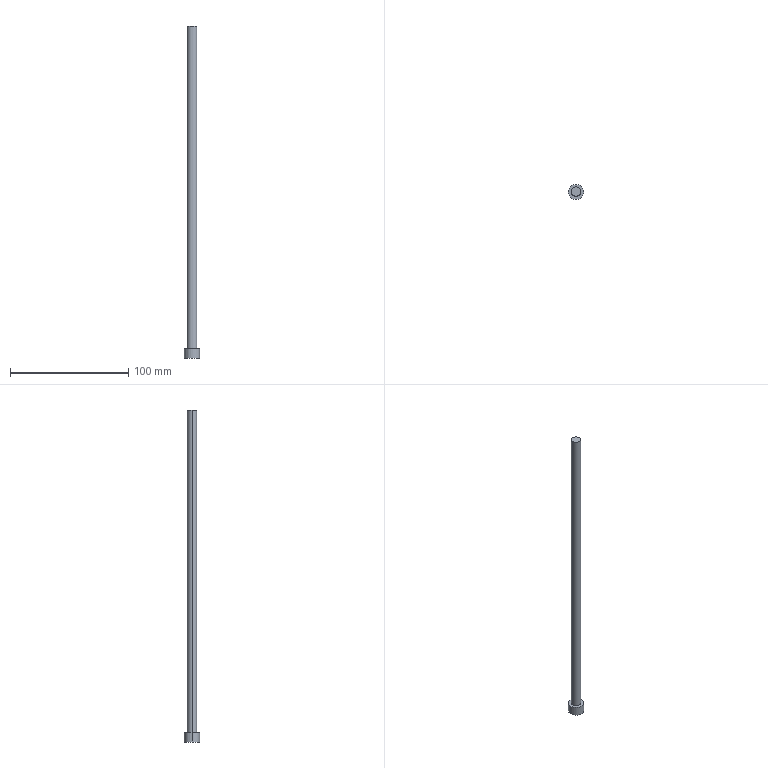Part | Creo | 1 solid | 7 faces | box 13 x 13 x 280.905 mm | volume 14780 mm3 | cylinder 4 | plane 3 | commonest cylinder face diameters 8 x2 13 x2
STEP:
#1=CARTESIAN_POINT('',(85.,64.,20.405));
#2=VERTEX_POINT('',#1);
#3=CARTESIAN_POINT('',(77.,64.,20.405));
#4=VERTEX_POINT('',#3);
#5=CARTESIAN_POINT('',(81.,64.,20.405));
#6=DIRECTION('',(0.,0.,1.));
#7=DIRECTION('',(1.,0.,0.));
#8=AXIS2_PLACEMENT_3D('',#5,#6,#7);
#9=CIRCLE('',#8,4.);
#10=EDGE_CURVE('',#2,#4,#9,.T.);
#11=ORIENTED_EDGE('',*,*,#10,.F.);
#12=CARTESIAN_POINT('',(81.,64.,20.405));
#13=DIRECTION('',(0.,0.,1.));
#14=DIRECTION('',(-1.,0.,0.));
#15=AXIS2_PLACEMENT_3D('',#12,#13,#14);
#16=CIRCLE('',#15,4.);
#17=EDGE_CURVE('',#4,#2,#16,.T.);
#18=ORIENTED_EDGE('',*,*,#17,.F.);
#19=EDGE_LOOP('',(#11,#18));
#20=FACE_OUTER_BOUND('',#19,.F.);
#21=CARTESIAN_POINT('',(81.,64.,20.405));
#22=DIRECTION('',(0.,0.,1.));
#23=DIRECTION('',(1.,0.,0.));
#24=AXIS2_PLACEMENT_3D('',#21,#22,#23);
#25=PLANE('',#24);
#26=ADVANCED_FACE('',(#20),#25,.T.);
#27=CARTESIAN_POINT('',(77.,64.,-252.5));
#28=VERTEX_POINT('',#27);
#29=CARTESIAN_POINT('',(85.,64.,-252.5));
#30=VERTEX_POINT('',#29);
#31=CARTESIAN_POINT('',(81.,64.,-252.5));
#32=DIRECTION('',(0.,0.,-1.));
#33=DIRECTION('',(-1.,0.,0.));
#34=AXIS2_PLACEMENT_3D('',#31,#32,#33);
#35=CIRCLE('',#34,4.);
#36=EDGE_CURVE('',#28,#30,#35,.T.);
#37=ORIENTED_EDGE('',*,*,#36,.T.);
#38=CARTESIAN_POINT('',(85.,64.,-252.5));
#39=DIRECTION('',(0.,0.,1.));
#40=VECTOR('',#39,272.905);
#41=LINE('',#38,#40);
#42=EDGE_CURVE('',#30,#2,#41,.T.);
#43=ORIENTED_EDGE('',*,*,#42,.T.);
#44=ORIENTED_EDGE('',*,*,#10,.T.);
#45=CARTESIAN_POINT('',(77.,64.,-252.5));
#46=DIRECTION('',(0.,0.,1.));
#47=VECTOR('',#46,272.905);
#48=LINE('',#45,#47);
#49=EDGE_CURVE('',#28,#4,#48,.T.);
#50=ORIENTED_EDGE('',*,*,#49,.F.);
#51=EDGE_LOOP('',(#37,#43,#44,#50));
#52=FACE_OUTER_BOUND('',#51,.F.);
#53=CARTESIAN_POINT('',(81.,64.,-255.5));
#54=DIRECTION('',(0.,0.,1.));
#55=DIRECTION('',(1.,0.,0.));
#56=AXIS2_PLACEMENT_3D('',#53,#54,#55);
#57=CYLINDRICAL_SURFACE('',#56,4.);
#58=ADVANCED_FACE('',(#52),#57,.T.);
#59=CARTESIAN_POINT('',(74.5,64.,-252.5));
#60=VERTEX_POINT('',#59);
#61=CARTESIAN_POINT('',(87.5,64.,-252.5));
#62=VERTEX_POINT('',#61);
#63=CARTESIAN_POINT('',(81.,64.,-252.5));
#64=DIRECTION('',(0.,0.,1.));
#65=DIRECTION('',(-1.,0.,0.));
#66=AXIS2_PLACEMENT_3D('',#63,#64,#65);
#67=CIRCLE('',#66,6.5);
#68=EDGE_CURVE('',#60,#62,#67,.T.);
#69=ORIENTED_EDGE('',*,*,#68,.F.);
#70=CARTESIAN_POINT('',(81.,64.,-252.5));
#71=DIRECTION('',(0.,0.,1.));
#72=DIRECTION('',(1.,0.,0.));
#73=AXIS2_PLACEMENT_3D('',#70,#71,#72);
#74=CIRCLE('',#73,6.5);
#75=EDGE_CURVE('',#62,#60,#74,.T.);
#76=ORIENTED_EDGE('',*,*,#75,.F.);
#77=EDGE_LOOP('',(#69,#76));
#78=FACE_OUTER_BOUND('',#77,.F.);
#79=CARTESIAN_POINT('',(81.,64.,-252.5));
#80=DIRECTION('',(0.,0.,-1.));
#81=DIRECTION('',(1.,0.,0.));
#82=AXIS2_PLACEMENT_3D('',#79,#80,#81);
#83=CIRCLE('',#82,4.);
#84=EDGE_CURVE('',#30,#28,#83,.T.);
#85=ORIENTED_EDGE('',*,*,#84,.F.);
#86=ORIENTED_EDGE('',*,*,#36,.F.);
#87=EDGE_LOOP('',(#85,#86));
#88=FACE_BOUND('',#87,.F.);
#89=CARTESIAN_POINT('',(81.,64.,-252.5));
#90=DIRECTION('',(0.,0.,1.));
#91=DIRECTION('',(1.,0.,0.));
#92=AXIS2_PLACEMENT_3D('',#89,#90,#91);
#93=PLANE('',#92);
#94=ADVANCED_FACE('',(#78,#88),#93,.T.);
#95=ORIENTED_EDGE('',*,*,#84,.T.);
#96=ORIENTED_EDGE('',*,*,#49,.T.);
#97=ORIENTED_EDGE('',*,*,#17,.T.);
#98=ORIENTED_EDGE('',*,*,#42,.F.);
#99=EDGE_LOOP('',(#95,#96,#97,#98));
#100=FACE_OUTER_BOUND('',#99,.F.);
#101=CARTESIAN_POINT('',(81.,64.,-255.5));
#102=DIRECTION('',(0.,0.,1.));
#103=DIRECTION('',(1.,0.,0.));
#104=AXIS2_PLACEMENT_3D('',#101,#102,#103);
#105=CYLINDRICAL_SURFACE('',#104,4.);
#106=ADVANCED_FACE('',(#100),#105,.T.);
#107=ORIENTED_EDGE('',*,*,#68,.T.);
#108=CARTESIAN_POINT('',(87.5,64.,-260.5));
#109=VERTEX_POINT('',#108);
#110=CARTESIAN_POINT('',(87.5,64.,-260.5));
#111=DIRECTION('',(0.,0.,1.));
#112=VECTOR('',#111,8.);
#113=LINE('',#110,#112);
#114=EDGE_CURVE('',#109,#62,#113,.T.);
#115=ORIENTED_EDGE('',*,*,#114,.F.);
#116=CARTESIAN_POINT('',(74.5,64.,-260.5));
#117=VERTEX_POINT('',#116);
#118=CARTESIAN_POINT('',(81.,64.,-260.5));
#119=DIRECTION('',(0.,0.,-1.));
#120=DIRECTION('',(1.,0.,0.));
#121=AXIS2_PLACEMENT_3D('',#118,#119,#120);
#122=CIRCLE('',#121,6.5);
#123=EDGE_CURVE('',#109,#117,#122,.T.);
#124=ORIENTED_EDGE('',*,*,#123,.T.);
#125=CARTESIAN_POINT('',(74.5,64.,-260.5));
#126=DIRECTION('',(0.,0.,1.));
#127=VECTOR('',#126,8.);
#128=LINE('',#125,#127);
#129=EDGE_CURVE('',#117,#60,#128,.T.);
#130=ORIENTED_EDGE('',*,*,#129,.T.);
#131=EDGE_LOOP('',(#107,#115,#124,#130));
#132=FACE_OUTER_BOUND('',#131,.F.);
#133=CARTESIAN_POINT('',(81.,64.,-260.5));
#134=DIRECTION('',(0.,0.,1.));
#135=DIRECTION('',(1.,0.,0.));
#136=AXIS2_PLACEMENT_3D('',#133,#134,#135);
#137=CYLINDRICAL_SURFACE('',#136,6.5);
#138=ADVANCED_FACE('',(#132),#137,.T.);
#139=ORIENTED_EDGE('',*,*,#75,.T.);
#140=ORIENTED_EDGE('',*,*,#129,.F.);
#141=CARTESIAN_POINT('',(81.,64.,-260.5));
#142=DIRECTION('',(0.,0.,-1.));
#143=DIRECTION('',(-1.,0.,0.));
#144=AXIS2_PLACEMENT_3D('',#141,#142,#143);
#145=CIRCLE('',#144,6.5);
#146=EDGE_CURVE('',#117,#109,#145,.T.);
#147=ORIENTED_EDGE('',*,*,#146,.T.);
#148=ORIENTED_EDGE('',*,*,#114,.T.);
#149=EDGE_LOOP('',(#139,#140,#147,#148));
#150=FACE_OUTER_BOUND('',#149,.F.);
#151=CARTESIAN_POINT('',(81.,64.,-260.5));
#152=DIRECTION('',(0.,0.,1.));
#153=DIRECTION('',(1.,0.,0.));
#154=AXIS2_PLACEMENT_3D('',#151,#152,#153);
#155=CYLINDRICAL_SURFACE('',#154,6.5);
#156=ADVANCED_FACE('',(#150),#155,.T.);
#157=ORIENTED_EDGE('',*,*,#123,.F.);
#158=ORIENTED_EDGE('',*,*,#146,.F.);
#159=EDGE_LOOP('',(#157,#158));
#160=FACE_OUTER_BOUND('',#159,.F.);
#161=CARTESIAN_POINT('',(81.,64.,-260.5));
#162=DIRECTION('',(0.,0.,-1.));
#163=DIRECTION('',(-1.,0.,0.));
#164=AXIS2_PLACEMENT_3D('',#161,#162,#163);
#165=PLANE('',#164);
#166=ADVANCED_FACE('',(#160),#165,.T.);
#167=CLOSED_SHELL('',(#26,#58,#94,#106,#138,#156,#166));
#168=MANIFOLD_SOLID_BREP('',#167);
#169=(LENGTH_UNIT()NAMED_UNIT(*)SI_UNIT(.MILLI.,.METRE.));
#170=UNCERTAINTY_MEASURE_WITH_UNIT(LENGTH_MEASURE(0.02815),#169,'','');
#171=(NAMED_UNIT(*)PLANE_ANGLE_UNIT()SI_UNIT($,.RADIAN.));
#172=PLANE_ANGLE_MEASURE_WITH_UNIT(PLANE_ANGLE_MEASURE(0.01745),#171);
#173=(CONVERSION_BASED_UNIT('DEGREE',#172)NAMED_UNIT(*)PLANE_ANGLE_UNIT());
#174=(NAMED_UNIT(*)SI_UNIT($,.STERADIAN.)SOLID_ANGLE_UNIT());
#175=(GEOMETRIC_REPRESENTATION_CONTEXT(3)GLOBAL_UNCERTAINTY_ASSIGNED_CONTEXT((#170))GLOBAL_UNIT_ASSIGNED_CONTEXT((#169,#173,#174))REPRESENTATION_CONTEXT('',''));
#176=ADVANCED_BREP_SHAPE_REPRESENTATION('',(#168),#175);